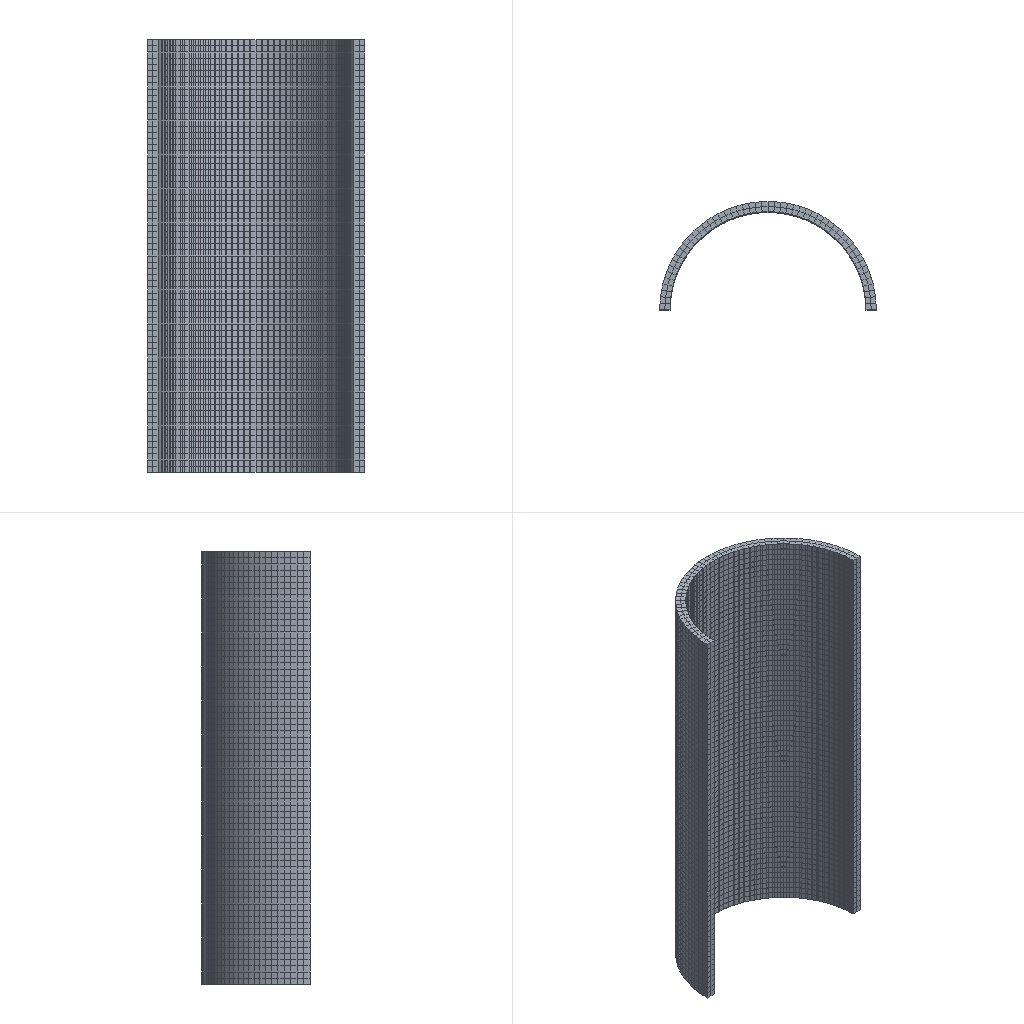Simulation study | abaqus
Set-up summary:
category,name,step,type,value,unit,region
solver,abaqus
solver,version,,,Abaqus/Explicit 2020
units,not stated in the deck,,not stated
analysis,deck,,transient,transient
load_step,Step-1,Step-1,transient,nlgeom=True
contact,interactions,,,general=1 pairs=0 ties=0
load_step,requested,,,1
mesh,nodes,,,18531
mesh,elements,,,10780
element_type,C3D8R,,solid,10780
load,load commands in deck,,count,1
bc,support commands in deck,,count,1
material,CON,,in results
material,STEEL,,in results
material,TNT,,in results
check,setup vs results,,match,"per instance, exact: element labels, types and connectivity; labels of the nodes the elements use; coordinates of those nodes at SINGLE_PRECISION in 2 of 2 instance(s)"
Abaqus input file, long lists of numbers shortened:
*Heading
** Job name: Job-1 Model name: Model-1
** Generated by: Abaqus/CAE 2020
*Preprint, echo=NO, model=NO, history=NO, contact=NO
**
** PARTS
**
*Part, name=P23051720-2
*Node
      1,   1.237,   1.237,         13.5
      2,   1.121,   1.121,         13.5
** (11287 more lines like these left out)
*Element, type=C3D8R
  1,  150, 1854, 8026, 1038,    1,   31, 1014,   56
  2, 1854,  185, 1446, 8026,   31,    2,   32, 1014
** (7278 more lines like these left out)
*Nset, nset=Set-1, generate
     1,  11289,      1
*Elset, elset=Set-1, generate
    1,  7280,     1
** Section: con
*Solid Section, elset=Set-1, material=con
,
*End Part
**
*Part, name=P23051720-5
*Node
      1,   1.583,           0.,          17.
      2,    1.58, 0.0994,          17.
** (7240 more lines like these left out)
*Element, type=C3D8R
   1, 3622, 3623, 3674, 3673,    1,    2,   53,   52
   2, 3623, 3624, 3675, 3674,    2,    3,   54,   53
** (3498 more lines like these left out)
*Nset, nset=Set-1, generate
    1,  7242,     1
*Elset, elset=Set-1, generate
    1,  3500,     1
*Nset, nset=Set-2, generate
    1,  7242,     1
*Elset, elset=Set-2, generate
    1,  3500,     1
*Nset, nset=Set-3, generate
    1,  7242,     1
*Elset, elset=Set-3, generate
    1,  3500,     1
** Section: s
*Solid Section, elset=Set-3, material=steel
,
*End Part
**
**
** ASSEMBLY
**
*Assembly, name=Assembly
**
*Instance, name=con, part=P23051720-2
          0.,        -2.98,        -13.5
*End Instance
**
*Instance, name=qiao, part=P23051720-5
          0.,        -2.98,        -13.5
*End Instance
**
*Node
      1,           0.,           0.,           0.
*Nset, nset=Set-2, instance=con
    5,    6,    7,    8,   11,   12,   17,   18,   19,   20,   21,   22,   23,   24,   25,   26
   27,   28,   29,   30,   57,   58,   59,   60,   61,   62,   63,   64,   65,   66,   67,   68
** (18 more lines like these left out)
*Nset, nset=Set-2, instance=qiao
    1,    2,    3,    4,    5,    6,    7,    8,    9,   10,   11,   12,   13,   14,   15,   16
   17,   18,   19,   20,   21,   22,   23,   24,   25,   26,   27,   28,   29,   30,   31,   32
** (11 more lines like these left out)
*Elset, elset=Set-2, instance=con
  885,  886,  887,  888,  889,  890,  891,  892,  893,  894,  895,  896,  897,  898,  899,  900
  901,  902,  903,  904,  905,  906,  907,  908,  909,  910, 1795, 1796, 1797, 1798, 1799, 1800
** (11 more lines like these left out)
*Elset, elset=Set-2, instance=qiao
    1,    2,    3,    4,    5,    6,    7,    8,    9,   10,   11,   12,   13,   14,   15,   16
   17,   18,   19,   20,   21,   22,   23,   24,   25,   26,   27,   28,   29,   30,   31,   32
** (5 more lines like these left out)
*Nset, nset=Set-3, instance=con
    3,    4,    6,    7,   14,   15,   17,   18,   23,   24,   28,   29,   44,   70,   83,   84
   85,   86,   87,   88,   89,   90,   91,   92,   93,   94,   95,   96,   97,   98,   99,  100
** (25 more lines like these left out)
*Nset, nset=Set-3, instance=qiao
    1,   51,   52,  102,  103,  153,  154,  204,  205,  255,  256,  306,  307,  357,  358,  408
  409,  459,  460,  510,  511,  561,  562,  612,  613,  663,  664,  714,  715,  765,  766,  816
** (16 more lines like these left out)
*Elset, elset=Set-3, instance=con
   25,   26,   51,   52,   77,   78,  103,  104,  129,  130,  155,  156,  181,  182,  207,  208
  233,  234,  259,  260,  285,  286,  311,  312,  337,  338,  363,  364,  389,  390,  415,  416
** (16 more lines like these left out)
*Elset, elset=Set-3, instance=qiao
    1,   50,   51,  100,  101,  150,  151,  200,  201,  250,  251,  300,  301,  350,  351,  400
  401,  450,  451,  500,  501,  550,  551,  600,  601,  650,  651,  700,  701,  750,  751,  800
** (7 more lines like these left out)
*Nset, nset=m_Set-1
 1,
*Elset, elset=_s_Surf-1_S6, internal, instance=con
    1,    3,    5,    7,    9,   11,   13,   15,   17,   19,   21,   23,   25,   27,   29,   31
   33,   35,   37,   39,   41,   43,   45,   47,   49,   51,   53,   55,   57,   59,   61,   63
** (112 more lines like these left out)
*Elset, elset=_s_Surf-1_S1, internal, instance=con
 5916, 5917, 5918, 5919, 5920, 5921, 5922, 5923, 5924, 5925, 5926, 5927, 5928, 5929, 5930, 5931
 5932, 5933, 5934, 5935, 5936, 5937, 5938, 5939, 5940, 5941, 5942, 5943, 5944, 5945, 5946, 5947
** (55 more lines like these left out)
*Elset, elset=_s_Surf-1_S3, internal, instance=con
 1821, 1822, 1823, 1824, 1825, 1826, 1827, 1828, 1829, 1830, 1831, 1832, 1833, 1847, 1848, 1849
 1850, 1851, 1852, 1853, 1854, 1855, 1856, 1857, 1858, 1859, 1873, 1874, 1875, 1876, 1877, 1878
** (55 more lines like these left out)
*Surface, type=ELEMENT, name=s_Surf-1
_s_Surf-1_S6, S6
_s_Surf-1_S1, S1
_s_Surf-1_S3, S3
*End Assembly
**
** MATERIALS
**
*Material, name=con
*Density
2400.,
*Elastic
 3.23e+10, 0.2
*Concrete Damaged Plasticity
30.,     0.1,    1.16, 0.6667,    0.05
*Concrete Compression Hardening
 1.08e+07,          0.
 1.79e+07, 8.06517e-05
  2.3e+07,  0.0002405
 2.59e+07, 0.0004695
 2.68e+07, 0.0007596
 2.61e+07,   0.001099
 2.36e+07,  0.001652
 1.91e+07,  0.002587
 1.56e+07,  0.003492
  1.3e+07,  0.004368
  1.1e+07,  0.005223
 9.57e+06,  0.006063
 8.43e+06,   0.006894
 7.53e+06,  0.007717
 6.79e+06,  0.008535
 6.18e+06,  0.009348
 5.67e+06,   0.01016
 5.24e+06,   0.01097
 4.54e+06,   0.01258
 4.01e+06,   0.01419
 3.58e+06,    0.01579
 2.96e+06,   0.01899
 2.51e+06,   0.02218
 2.19e+06,   0.02537
 1.94e+06,     0.02856
 1.74e+06,   0.03175
 1.38e+06,   0.03971
 1.14e+06,   0.04766
  977000.,   0.05562
  853000.,   0.06357
  757000.,   0.07153
  680000.,   0.07948
  565000.,   0.09538
  484000.,    0.1113
  423000.,    0.1272
  375000.,    0.1431
  337000.,     0.159
*Concrete Tension Stiffening
 2.39e+06,       0.
 2.31e+06, 1.73e-05
 2.11e+06, 4.56e-05
 1.81e+06,  9.2e-05
 1.58e+06, 0.000136
 1.41e+06, 0.000178
 1.28e+06, 0.000219
 1.18e+06,  0.00026
 1.09e+06, 0.000299
 1.02e+06, 0.000339
  958000., 0.000378
  905000., 0.000416
  860000., 0.000455
  819000., 0.000493
  752000., 0.000569
  697000., 0.000645
  651000.,  0.00072
  578000., 0.000871
  523000.,  0.00102
  480000.,  0.00117
  444000.,  0.00132
  415000.,  0.00147
  359000.,  0.00184
  318000.,  0.00221
  287000.,  0.00258
  263000.,  0.00295
  243000.,  0.00332
  227000.,   0.0037
  201000.,  0.00444
  181000.,  0.00518
  166000.,  0.00592
  153000.,  0.00666
  143000.,   0.0074
*Concrete Compression Damage
        0.,          0.
 0.06555, 8.06517e-05
  0.1352,  0.0002405
  0.2057, 0.0004695
  0.2773, 0.0007596
  0.3489,   0.001099
  0.4457,  0.001652
  0.5681,  0.002587
  0.6515,  0.003492
*concrete failure
0.00001,0,0,0
*Concrete Tension Damage
     0.,       0.
 0.0236, 1.73e-05
 0.0651, 4.56e-05
  0.141,  9.2e-05
  0.217, 0.000136
  0.289, 0.000178
  0.356, 0.000219
  0.416,  0.00026
   0.47, 0.000299
  0.518, 0.000339
   0.56, 0.000378
  0.597, 0.000416
  0.631, 0.000455
*Material, name=steel
*Density
7800.,
*Elastic
 2.1e+11, 0.3
*Plastic, hardening=JOHNSON COOK
 5e+08, 8.57e+08,  0.3426,    0.665,    1523.,      25.
*Rate Dependent, type=JOHNSON COOK
 0.0326,1.
*Material, name=tnt
*Density
1630.,
*Eos, type=JWL
6390., 3.738e+11, 3.747e+09,      0.35,      4.15,       0.9,   4.3e+06,   2.1e+10
*Detonation Point
0.,0.,0.,0.
**
** INTERACTION PROPERTIES
**
*Surface Interaction, name=IntProp-2
*Friction
 0.2,
*Surface Behavior, pressure-overclosure=HARD
*Incident Wave Interaction Property, name=IntProp-1, type=AIR BLAST
*CONWEP Charge Property
3000., 1.
1., 1., 1.
** ----------------------------------------------------------------
**
** STEP: Step-1
**
*Step, name=Step-1, nlgeom=YES
*Dynamic, Explicit
, 0.001
*Bulk Viscosity
0.06, 1.2
**
** BOUNDARY CONDITIONS
**
** Name: BC-1 Type: 对称/反对称/完全固定
*Boundary
Set-3, ENCASTRE
**
** INTERACTIONS
**
** Interaction: Int-1
*Incident Wave Interaction, CONWEP, property=IntProp-1
s_Surf-1, m_Set-1,   , 0., 1.
** Interaction: Int-2
*Contact, op=NEW
*Contact Inclusions, ALL EXTERIOR
*Contact Property Assignment
 ,  , IntProp-2
**
** OUTPUT REQUESTS
**
*Restart, write, number interval=1, time marks=NO
**
** FIELD OUTPUT: F-Output-1
**
*Output, field
*Node Output
A, CF, RF, RM, RT, U, V
*Element Output, directions=YES
DAMAGEC, DAMAGET, E, EVF, LE, MISES, MISESMAX, MISESONLY, PE, PEEQ, PEEQVAVG, PEMAG, PEVAVG, S, SDEG, SF
STATUS, SVAVG, YIELDPOT
*Contact Output
CDISP, CSTRESS
**
** HISTORY OUTPUT: H-Output-1
**
*Output, history, variable=PRESELECT
*End Step
Results summary:
result,step,Step-1,completed,increments=4141 time=0.001/0.001
result,analysis,,,transient
result,last_loadstep,,,1
result,analysis steps,,count,1
result,primary field,,,U
result,reaction total,,FX,43849.263,model units
result,reaction total,,FY,78979863.362,model units
result,reaction total,,FZ,-23068.401,model units